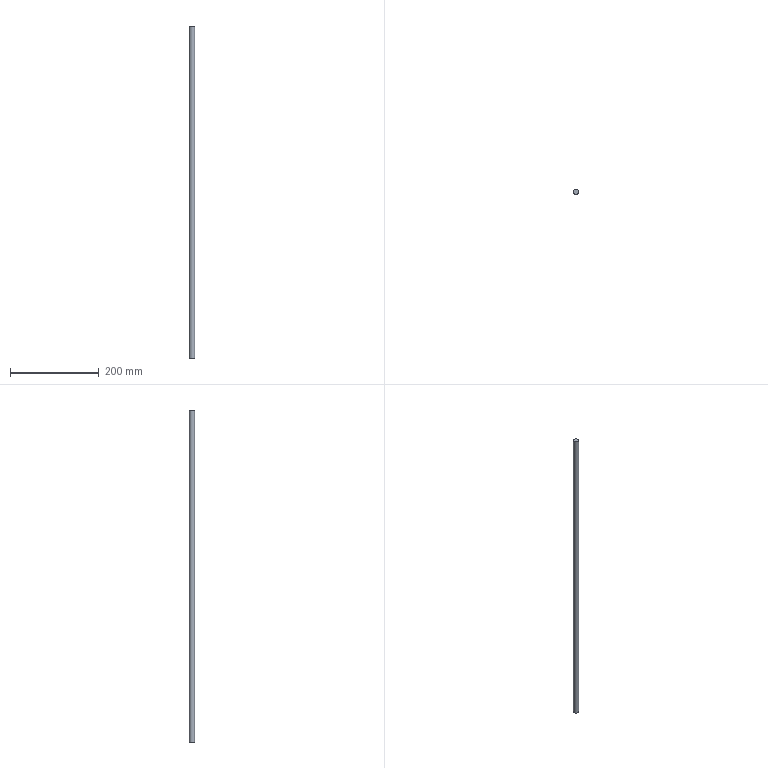Part | STEP file | 冲床-300配套压波_id502_x_t | 1 solid | 3 faces | box 12 x 12 x 750 mm | volume 84823 mm3 | plane 2 | cylinder 1 | commonest cylinder face diameters 12 x1
STEP:
#1=CARTESIAN_POINT('',(1143.,-119.,-25.));
#2=VERTEX_POINT('',#1);
#3=CARTESIAN_POINT('',(1137.,-119.,-25.));
#4=DIRECTION('',(0.,0.,1.));
#5=DIRECTION('',(1.,0.,0.));
#6=AXIS2_PLACEMENT_3D('',#3,#4,#5);
#7=CIRCLE('',#6,6.);
#8=EDGE_CURVE('',#2,#2,#7,.T.);
#9=ORIENTED_EDGE('',*,*,#8,.F.);
#10=EDGE_LOOP('',(#9));
#11=FACE_BOUND('',#10,.T.);
#12=CARTESIAN_POINT('',(1143.,-119.,-775.));
#13=VERTEX_POINT('',#12);
#14=CARTESIAN_POINT('',(1137.,-119.,-775.));
#15=DIRECTION('',(0.,0.,1.));
#16=DIRECTION('',(1.,0.,0.));
#17=AXIS2_PLACEMENT_3D('',#14,#15,#16);
#18=CIRCLE('',#17,6.);
#19=EDGE_CURVE('',#13,#13,#18,.T.);
#20=ORIENTED_EDGE('',*,*,#19,.T.);
#21=EDGE_LOOP('',(#20));
#22=FACE_BOUND('',#21,.T.);
#23=CARTESIAN_POINT('',(1137.,-119.,-506.));
#24=DIRECTION('',(0.,0.,-1.));
#25=DIRECTION('',(1.,0.,0.));
#26=AXIS2_PLACEMENT_3D('',#23,#24,#25);
#27=CYLINDRICAL_SURFACE('',#26,6.);
#28=ADVANCED_FACE('',(#11,#22),#27,.T.);
#29=ORIENTED_EDGE('',*,*,#8,.T.);
#30=EDGE_LOOP('',(#29));
#31=FACE_OUTER_BOUND('',#30,.T.);
#32=CARTESIAN_POINT('',(1137.,-119.,-25.));
#33=DIRECTION('',(0.,0.,1.));
#34=DIRECTION('',(-1.,0.,0.));
#35=AXIS2_PLACEMENT_3D('',#32,#33,#34);
#36=PLANE('',#35);
#37=ADVANCED_FACE('',(#31),#36,.T.);
#38=ORIENTED_EDGE('',*,*,#19,.F.);
#39=EDGE_LOOP('',(#38));
#40=FACE_OUTER_BOUND('',#39,.T.);
#41=CARTESIAN_POINT('',(1137.,-119.,-775.));
#42=DIRECTION('',(0.,0.,1.));
#43=DIRECTION('',(-1.,0.,0.));
#44=AXIS2_PLACEMENT_3D('',#41,#42,#43);
#45=PLANE('',#44);
#46=ADVANCED_FACE('',(#40),#45,.F.);
#47=CLOSED_SHELL('',(#28,#37,#46));
#48=MANIFOLD_SOLID_BREP('',#47);
#49=(LENGTH_UNIT()NAMED_UNIT(*)SI_UNIT(.MILLI.,.METRE.));
#50=UNCERTAINTY_MEASURE_WITH_UNIT(LENGTH_MEASURE(0.00002),#49,'','');
#51=(NAMED_UNIT(*)PLANE_ANGLE_UNIT()SI_UNIT($,.RADIAN.));
#52=PLANE_ANGLE_MEASURE_WITH_UNIT(PLANE_ANGLE_MEASURE(0.01745),#51);
#53=DIMENSIONAL_EXPONENTS(0.,0.,0.,0.,0.,0.,0.);
#54=(CONVERSION_BASED_UNIT('DEGREE',#52)NAMED_UNIT(#53)PLANE_ANGLE_UNIT());
#55=(NAMED_UNIT(*)SI_UNIT($,.STERADIAN.)SOLID_ANGLE_UNIT());
#56=(GEOMETRIC_REPRESENTATION_CONTEXT(3)GLOBAL_UNCERTAINTY_ASSIGNED_CONTEXT((#50))GLOBAL_UNIT_ASSIGNED_CONTEXT((#49,#54,#55))REPRESENTATION_CONTEXT('',''));
#57=ADVANCED_BREP_SHAPE_REPRESENTATION('',(#48),#56);